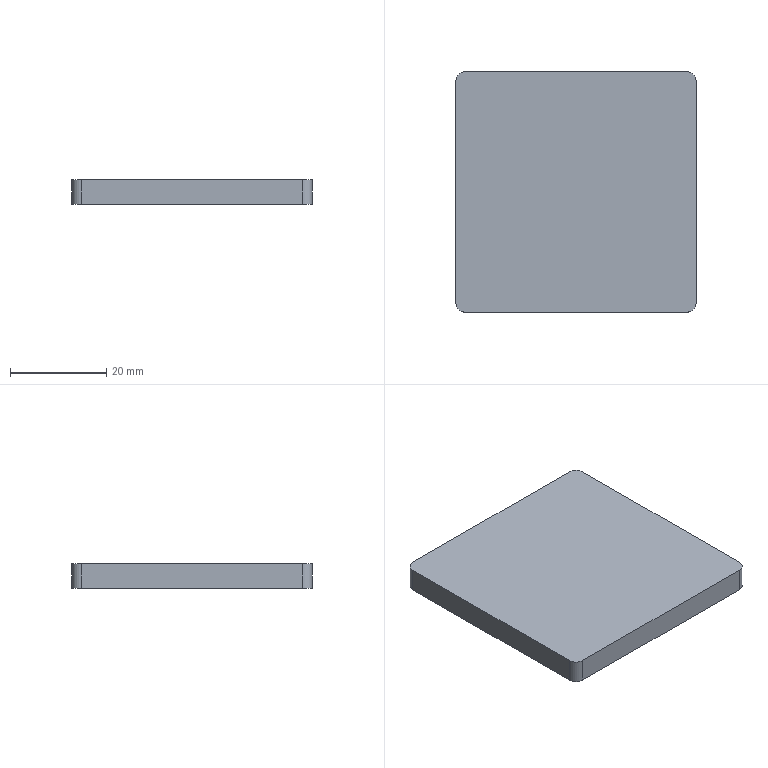Part | SolidWorks | features Fillet 2, ICE 2, Extrusion 1 | 1 solid | 10 faces | box 50 x 50 x 5 mm | volume 12483 mm3 | plane 6 | cylinder 4 | commonest cylinder face diameters 4 x4
STEP:
#1=CARTESIAN_POINT('',(-23.,-25.,0.));
#2=VERTEX_POINT('',#1);
#3=CARTESIAN_POINT('',(-25.,-23.,0.));
#4=VERTEX_POINT('',#3);
#5=CARTESIAN_POINT('',(-23.,-23.,0.));
#6=DIRECTION('',(0.,0.,-1.));
#7=DIRECTION('',(-1.,0.,0.));
#8=AXIS2_PLACEMENT_3D('',#5,#6,#7);
#9=CIRCLE('',#8,2.);
#10=EDGE_CURVE('',#2,#4,#9,.T.);
#11=ORIENTED_EDGE('',*,*,#10,.T.);
#12=CARTESIAN_POINT('',(-25.,-23.,-5.));
#13=VERTEX_POINT('',#12);
#14=CARTESIAN_POINT('',(-25.,-23.,-5.));
#15=DIRECTION('',(0.,0.,1.));
#16=VECTOR('',#15,1000.);
#17=LINE('',#14,#16);
#18=EDGE_CURVE('',#13,#4,#17,.T.);
#19=ORIENTED_EDGE('',*,*,#18,.F.);
#20=CARTESIAN_POINT('',(-23.,-25.,-5.));
#21=VERTEX_POINT('',#20);
#22=CARTESIAN_POINT('',(-23.,-23.,-5.));
#23=DIRECTION('',(0.,0.,-1.));
#24=DIRECTION('',(-1.,0.,0.));
#25=AXIS2_PLACEMENT_3D('',#22,#23,#24);
#26=CIRCLE('',#25,2.);
#27=EDGE_CURVE('',#21,#13,#26,.T.);
#28=ORIENTED_EDGE('',*,*,#27,.F.);
#29=CARTESIAN_POINT('',(-23.,-25.,-5.));
#30=DIRECTION('',(0.,0.,1.));
#31=VECTOR('',#30,1000.);
#32=LINE('',#29,#31);
#33=EDGE_CURVE('',#21,#2,#32,.T.);
#34=ORIENTED_EDGE('',*,*,#33,.T.);
#35=EDGE_LOOP('',(#11,#19,#28,#34));
#36=FACE_OUTER_BOUND('',#35,.T.);
#37=CARTESIAN_POINT('',(-23.,-23.,-5.));
#38=DIRECTION('',(0.,0.,1.));
#39=DIRECTION('',(1.,0.,0.));
#40=AXIS2_PLACEMENT_3D('',#37,#38,#39);
#41=CYLINDRICAL_SURFACE('',#40,2.);
#42=ADVANCED_FACE('',(#36),#41,.T.);
#43=CARTESIAN_POINT('',(-25.,23.,0.));
#44=VERTEX_POINT('',#43);
#45=CARTESIAN_POINT('',(-25.,23.,0.));
#46=DIRECTION('',(0.,1.,0.));
#47=VECTOR('',#46,1000.);
#48=LINE('',#45,#47);
#49=EDGE_CURVE('',#4,#44,#48,.T.);
#50=ORIENTED_EDGE('',*,*,#49,.T.);
#51=CARTESIAN_POINT('',(-25.,23.,-5.));
#52=VERTEX_POINT('',#51);
#53=CARTESIAN_POINT('',(-25.,23.,-5.));
#54=DIRECTION('',(0.,0.,1.));
#55=VECTOR('',#54,1000.);
#56=LINE('',#53,#55);
#57=EDGE_CURVE('',#52,#44,#56,.T.);
#58=ORIENTED_EDGE('',*,*,#57,.F.);
#59=CARTESIAN_POINT('',(-25.,23.,-5.));
#60=DIRECTION('',(0.,1.,0.));
#61=VECTOR('',#60,1000.);
#62=LINE('',#59,#61);
#63=EDGE_CURVE('',#13,#52,#62,.T.);
#64=ORIENTED_EDGE('',*,*,#63,.F.);
#65=ORIENTED_EDGE('',*,*,#18,.T.);
#66=EDGE_LOOP('',(#50,#58,#64,#65));
#67=FACE_OUTER_BOUND('',#66,.T.);
#68=CARTESIAN_POINT('',(-25.,23.,-5.));
#69=DIRECTION('',(1.,0.,0.));
#70=DIRECTION('',(0.,0.,-1.));
#71=AXIS2_PLACEMENT_3D('',#68,#69,#70);
#72=PLANE('',#71);
#73=ADVANCED_FACE('',(#67),#72,.F.);
#74=CARTESIAN_POINT('',(-23.,25.,0.));
#75=VERTEX_POINT('',#74);
#76=CARTESIAN_POINT('',(-23.,23.,0.));
#77=DIRECTION('',(0.,0.,-1.));
#78=DIRECTION('',(-1.,0.,0.));
#79=AXIS2_PLACEMENT_3D('',#76,#77,#78);
#80=CIRCLE('',#79,2.);
#81=EDGE_CURVE('',#44,#75,#80,.T.);
#82=ORIENTED_EDGE('',*,*,#81,.T.);
#83=CARTESIAN_POINT('',(-23.,25.,-5.));
#84=VERTEX_POINT('',#83);
#85=CARTESIAN_POINT('',(-23.,25.,-5.));
#86=DIRECTION('',(0.,0.,1.));
#87=VECTOR('',#86,1000.);
#88=LINE('',#85,#87);
#89=EDGE_CURVE('',#84,#75,#88,.T.);
#90=ORIENTED_EDGE('',*,*,#89,.F.);
#91=CARTESIAN_POINT('',(-23.,23.,-5.));
#92=DIRECTION('',(0.,0.,-1.));
#93=DIRECTION('',(-1.,0.,0.));
#94=AXIS2_PLACEMENT_3D('',#91,#92,#93);
#95=CIRCLE('',#94,2.);
#96=EDGE_CURVE('',#52,#84,#95,.T.);
#97=ORIENTED_EDGE('',*,*,#96,.F.);
#98=ORIENTED_EDGE('',*,*,#57,.T.);
#99=EDGE_LOOP('',(#82,#90,#97,#98));
#100=FACE_OUTER_BOUND('',#99,.T.);
#101=CARTESIAN_POINT('',(-23.,23.,-5.));
#102=DIRECTION('',(0.,0.,1.));
#103=DIRECTION('',(1.,0.,0.));
#104=AXIS2_PLACEMENT_3D('',#101,#102,#103);
#105=CYLINDRICAL_SURFACE('',#104,2.);
#106=ADVANCED_FACE('',(#100),#105,.T.);
#107=CARTESIAN_POINT('',(23.,25.,0.));
#108=VERTEX_POINT('',#107);
#109=CARTESIAN_POINT('',(23.,25.,0.));
#110=DIRECTION('',(1.,0.,0.));
#111=VECTOR('',#110,1000.);
#112=LINE('',#109,#111);
#113=EDGE_CURVE('',#75,#108,#112,.T.);
#114=ORIENTED_EDGE('',*,*,#113,.T.);
#115=CARTESIAN_POINT('',(23.,25.,-5.));
#116=VERTEX_POINT('',#115);
#117=CARTESIAN_POINT('',(23.,25.,-5.));
#118=DIRECTION('',(0.,0.,1.));
#119=VECTOR('',#118,1000.);
#120=LINE('',#117,#119);
#121=EDGE_CURVE('',#116,#108,#120,.T.);
#122=ORIENTED_EDGE('',*,*,#121,.F.);
#123=CARTESIAN_POINT('',(23.,25.,-5.));
#124=DIRECTION('',(1.,0.,0.));
#125=VECTOR('',#124,1000.);
#126=LINE('',#123,#125);
#127=EDGE_CURVE('',#84,#116,#126,.T.);
#128=ORIENTED_EDGE('',*,*,#127,.F.);
#129=ORIENTED_EDGE('',*,*,#89,.T.);
#130=EDGE_LOOP('',(#114,#122,#128,#129));
#131=FACE_OUTER_BOUND('',#130,.T.);
#132=CARTESIAN_POINT('',(23.,25.,-5.));
#133=DIRECTION('',(0.,-1.,0.));
#134=DIRECTION('',(0.,0.,-1.));
#135=AXIS2_PLACEMENT_3D('',#132,#133,#134);
#136=PLANE('',#135);
#137=ADVANCED_FACE('',(#131),#136,.F.);
#138=CARTESIAN_POINT('',(25.,23.,0.));
#139=VERTEX_POINT('',#138);
#140=CARTESIAN_POINT('',(23.,23.,0.));
#141=DIRECTION('',(0.,0.,-1.));
#142=DIRECTION('',(-1.,0.,0.));
#143=AXIS2_PLACEMENT_3D('',#140,#141,#142);
#144=CIRCLE('',#143,2.);
#145=EDGE_CURVE('',#108,#139,#144,.T.);
#146=ORIENTED_EDGE('',*,*,#145,.T.);
#147=CARTESIAN_POINT('',(25.,23.,-5.));
#148=VERTEX_POINT('',#147);
#149=CARTESIAN_POINT('',(25.,23.,-5.));
#150=DIRECTION('',(0.,0.,1.));
#151=VECTOR('',#150,1000.);
#152=LINE('',#149,#151);
#153=EDGE_CURVE('',#148,#139,#152,.T.);
#154=ORIENTED_EDGE('',*,*,#153,.F.);
#155=CARTESIAN_POINT('',(23.,23.,-5.));
#156=DIRECTION('',(0.,0.,-1.));
#157=DIRECTION('',(-1.,0.,0.));
#158=AXIS2_PLACEMENT_3D('',#155,#156,#157);
#159=CIRCLE('',#158,2.);
#160=EDGE_CURVE('',#116,#148,#159,.T.);
#161=ORIENTED_EDGE('',*,*,#160,.F.);
#162=ORIENTED_EDGE('',*,*,#121,.T.);
#163=EDGE_LOOP('',(#146,#154,#161,#162));
#164=FACE_OUTER_BOUND('',#163,.T.);
#165=CARTESIAN_POINT('',(23.,23.,-5.));
#166=DIRECTION('',(0.,0.,1.));
#167=DIRECTION('',(1.,0.,0.));
#168=AXIS2_PLACEMENT_3D('',#165,#166,#167);
#169=CYLINDRICAL_SURFACE('',#168,2.);
#170=ADVANCED_FACE('',(#164),#169,.T.);
#171=CARTESIAN_POINT('',(25.,-23.,0.));
#172=VERTEX_POINT('',#171);
#173=CARTESIAN_POINT('',(25.,-23.,0.));
#174=DIRECTION('',(0.,-1.,0.));
#175=VECTOR('',#174,1000.);
#176=LINE('',#173,#175);
#177=EDGE_CURVE('',#139,#172,#176,.T.);
#178=ORIENTED_EDGE('',*,*,#177,.T.);
#179=CARTESIAN_POINT('',(25.,-23.,-5.));
#180=VERTEX_POINT('',#179);
#181=CARTESIAN_POINT('',(25.,-23.,-5.));
#182=DIRECTION('',(0.,0.,1.));
#183=VECTOR('',#182,1000.);
#184=LINE('',#181,#183);
#185=EDGE_CURVE('',#180,#172,#184,.T.);
#186=ORIENTED_EDGE('',*,*,#185,.F.);
#187=CARTESIAN_POINT('',(25.,-23.,-5.));
#188=DIRECTION('',(0.,-1.,0.));
#189=VECTOR('',#188,1000.);
#190=LINE('',#187,#189);
#191=EDGE_CURVE('',#148,#180,#190,.T.);
#192=ORIENTED_EDGE('',*,*,#191,.F.);
#193=ORIENTED_EDGE('',*,*,#153,.T.);
#194=EDGE_LOOP('',(#178,#186,#192,#193));
#195=FACE_OUTER_BOUND('',#194,.T.);
#196=CARTESIAN_POINT('',(25.,-23.,-5.));
#197=DIRECTION('',(-1.,0.,0.));
#198=DIRECTION('',(0.,0.,1.));
#199=AXIS2_PLACEMENT_3D('',#196,#197,#198);
#200=PLANE('',#199);
#201=ADVANCED_FACE('',(#195),#200,.F.);
#202=CARTESIAN_POINT('',(23.,-25.,0.));
#203=VERTEX_POINT('',#202);
#204=CARTESIAN_POINT('',(23.,-23.,0.));
#205=DIRECTION('',(0.,0.,-1.));
#206=DIRECTION('',(-1.,0.,0.));
#207=AXIS2_PLACEMENT_3D('',#204,#205,#206);
#208=CIRCLE('',#207,2.);
#209=EDGE_CURVE('',#172,#203,#208,.T.);
#210=ORIENTED_EDGE('',*,*,#209,.T.);
#211=CARTESIAN_POINT('',(23.,-25.,-5.));
#212=VERTEX_POINT('',#211);
#213=CARTESIAN_POINT('',(23.,-25.,-5.));
#214=DIRECTION('',(0.,0.,1.));
#215=VECTOR('',#214,1000.);
#216=LINE('',#213,#215);
#217=EDGE_CURVE('',#212,#203,#216,.T.);
#218=ORIENTED_EDGE('',*,*,#217,.F.);
#219=CARTESIAN_POINT('',(23.,-23.,-5.));
#220=DIRECTION('',(0.,0.,-1.));
#221=DIRECTION('',(-1.,0.,0.));
#222=AXIS2_PLACEMENT_3D('',#219,#220,#221);
#223=CIRCLE('',#222,2.);
#224=EDGE_CURVE('',#180,#212,#223,.T.);
#225=ORIENTED_EDGE('',*,*,#224,.F.);
#226=ORIENTED_EDGE('',*,*,#185,.T.);
#227=EDGE_LOOP('',(#210,#218,#225,#226));
#228=FACE_OUTER_BOUND('',#227,.T.);
#229=CARTESIAN_POINT('',(23.,-23.,-5.));
#230=DIRECTION('',(0.,0.,1.));
#231=DIRECTION('',(1.,0.,0.));
#232=AXIS2_PLACEMENT_3D('',#229,#230,#231);
#233=CYLINDRICAL_SURFACE('',#232,2.);
#234=ADVANCED_FACE('',(#228),#233,.T.);
#235=CARTESIAN_POINT('',(-23.,-25.,0.));
#236=DIRECTION('',(-1.,0.,0.));
#237=VECTOR('',#236,1000.);
#238=LINE('',#235,#237);
#239=EDGE_CURVE('',#203,#2,#238,.T.);
#240=ORIENTED_EDGE('',*,*,#239,.T.);
#241=ORIENTED_EDGE('',*,*,#33,.F.);
#242=CARTESIAN_POINT('',(-23.,-25.,-5.));
#243=DIRECTION('',(-1.,0.,0.));
#244=VECTOR('',#243,1000.);
#245=LINE('',#242,#244);
#246=EDGE_CURVE('',#212,#21,#245,.T.);
#247=ORIENTED_EDGE('',*,*,#246,.F.);
#248=ORIENTED_EDGE('',*,*,#217,.T.);
#249=EDGE_LOOP('',(#240,#241,#247,#248));
#250=FACE_OUTER_BOUND('',#249,.T.);
#251=CARTESIAN_POINT('',(-23.,-25.,-5.));
#252=DIRECTION('',(0.,1.,0.));
#253=DIRECTION('',(0.,0.,1.));
#254=AXIS2_PLACEMENT_3D('',#251,#252,#253);
#255=PLANE('',#254);
#256=ADVANCED_FACE('',(#250),#255,.F.);
#257=ORIENTED_EDGE('',*,*,#27,.T.);
#258=ORIENTED_EDGE('',*,*,#63,.T.);
#259=ORIENTED_EDGE('',*,*,#96,.T.);
#260=ORIENTED_EDGE('',*,*,#127,.T.);
#261=ORIENTED_EDGE('',*,*,#160,.T.);
#262=ORIENTED_EDGE('',*,*,#191,.T.);
#263=ORIENTED_EDGE('',*,*,#224,.T.);
#264=ORIENTED_EDGE('',*,*,#246,.T.);
#265=EDGE_LOOP('',(#257,#258,#259,#260,#261,#262,#263,#264));
#266=FACE_OUTER_BOUND('',#265,.T.);
#267=CARTESIAN_POINT('',(-23.,-23.,-5.));
#268=DIRECTION('',(0.,0.,-1.));
#269=DIRECTION('',(-1.,0.,0.));
#270=AXIS2_PLACEMENT_3D('',#267,#268,#269);
#271=PLANE('',#270);
#272=ADVANCED_FACE('',(#266),#271,.T.);
#273=ORIENTED_EDGE('',*,*,#10,.F.);
#274=ORIENTED_EDGE('',*,*,#239,.F.);
#275=ORIENTED_EDGE('',*,*,#209,.F.);
#276=ORIENTED_EDGE('',*,*,#177,.F.);
#277=ORIENTED_EDGE('',*,*,#145,.F.);
#278=ORIENTED_EDGE('',*,*,#113,.F.);
#279=ORIENTED_EDGE('',*,*,#81,.F.);
#280=ORIENTED_EDGE('',*,*,#49,.F.);
#281=EDGE_LOOP('',(#273,#274,#275,#276,#277,#278,#279,#280));
#282=FACE_OUTER_BOUND('',#281,.T.);
#283=CARTESIAN_POINT('',(-23.,-23.,0.));
#284=DIRECTION('',(0.,0.,-1.));
#285=DIRECTION('',(-1.,0.,0.));
#286=AXIS2_PLACEMENT_3D('',#283,#284,#285);
#287=PLANE('',#286);
#288=ADVANCED_FACE('',(#282),#287,.F.);
#289=CLOSED_SHELL('',(#42,#73,#106,#137,#170,#201,#234,#256,#272,#288));
#290=MANIFOLD_SOLID_BREP('',#289);
#291=CARTESIAN_POINT('',(0.,0.,0.));
#292=DIRECTION('',(0.,0.,1.));
#293=DIRECTION('',(1.,0.,0.));
#294=AXIS2_PLACEMENT_3D('',#291,#292,#293);
#295=(LENGTH_UNIT()NAMED_UNIT(*)SI_UNIT(.MILLI.,.METRE.));
#296=UNCERTAINTY_MEASURE_WITH_UNIT(LENGTH_MEASURE(0.00001),#295,'','');
#297=(NAMED_UNIT(*)PLANE_ANGLE_UNIT()SI_UNIT($,.RADIAN.));
#298=(NAMED_UNIT(*)SI_UNIT($,.STERADIAN.)SOLID_ANGLE_UNIT());
#299=(GEOMETRIC_REPRESENTATION_CONTEXT(3)GLOBAL_UNCERTAINTY_ASSIGNED_CONTEXT((#296))GLOBAL_UNIT_ASSIGNED_CONTEXT((#295,#297,#298))REPRESENTATION_CONTEXT('',''));
#300=ADVANCED_BREP_SHAPE_REPRESENTATION('',(#290,#294),#299);